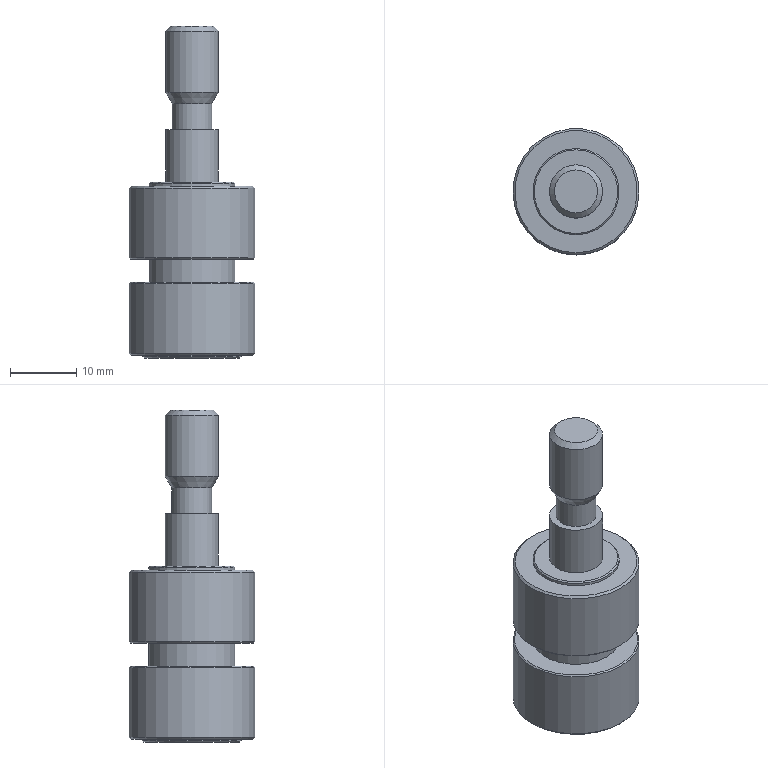Part | STEP file | 1 solid | 31 faces | box 19 x 19 x 50 mm | volume 7855 mm3 | plane 15 | cone 8 | cylinder 8 | commonest cylinder face diameters 8 x2 13 x2 19 x2 6 x1 14.9 x1